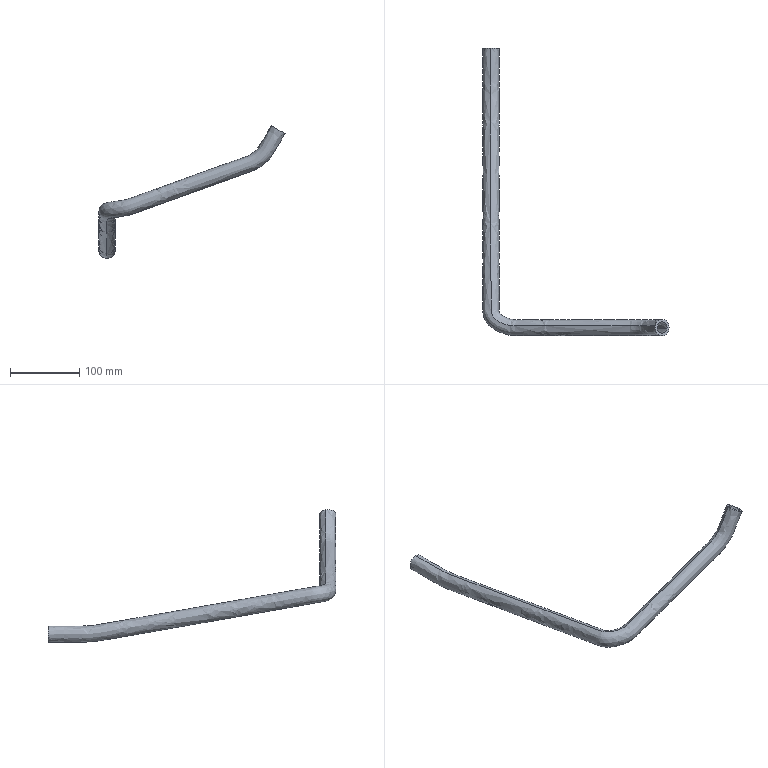Part | STEP file | ZXW722-L-57 | 1 solid | 6 faces | box 268.527 x 414.68 x 191.423 mm | volume 152673 mm3 | spline 4 | plane 2